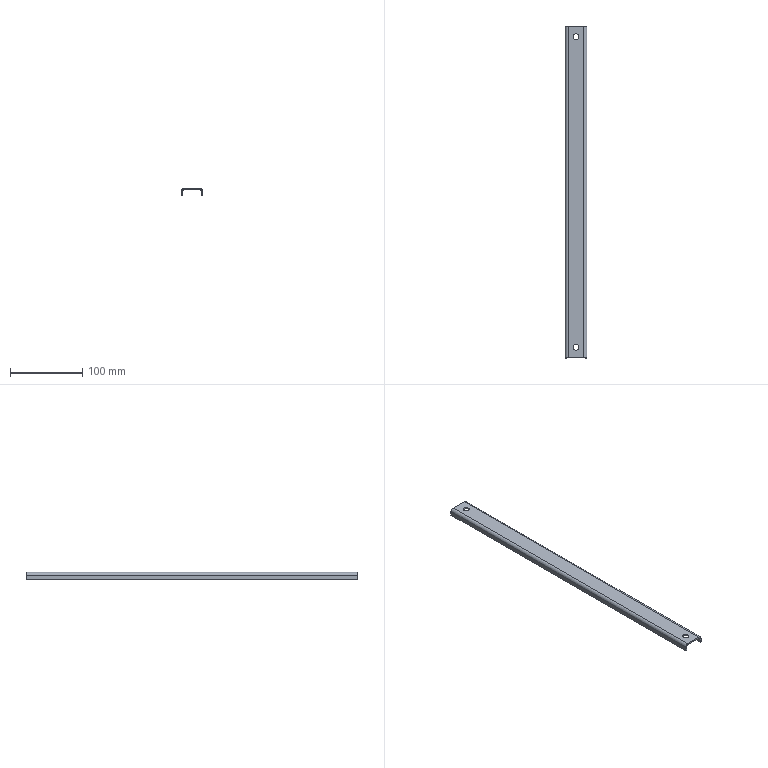Part | NX | features solid 2 | 1 solid | 18 faces | box 30 x 460 x 10 mm | volume 39740 mm3 | plane 10 | cylinder 8 | commonest cylinder face diameters 8.2 x4 4 x2 8 x2
STEP:
#1=CARTESIAN_POINT('',(690.9,502.5,-503.));
#2=VERTEX_POINT('',#1);
#3=CARTESIAN_POINT('',(690.9,502.5,-505.));
#4=VERTEX_POINT('',#3);
#5=CARTESIAN_POINT('',(690.9,502.5,-964.086));
#6=DIRECTION('',(0.,0.,1.));
#7=VECTOR('',#6,1000.);
#8=LINE('',#5,#7);
#9=EDGE_CURVE('',#2,#4,#8,.F.);
#10=ORIENTED_EDGE('',*,*,#9,.T.);
#11=CARTESIAN_POINT('',(699.1,502.5,-505.));
#12=VERTEX_POINT('',#11);
#13=CARTESIAN_POINT('',(695.,502.5,-505.));
#14=DIRECTION('',(0.,0.,-1.));
#15=DIRECTION('',(-1.,0.,0.));
#16=AXIS2_PLACEMENT_3D('',#13,#14,#15);
#17=CIRCLE('',#16,4.1);
#18=EDGE_CURVE('',#4,#12,#17,.T.);
#19=ORIENTED_EDGE('',*,*,#18,.T.);
#20=CARTESIAN_POINT('',(699.1,502.5,-503.));
#21=VERTEX_POINT('',#20);
#22=CARTESIAN_POINT('',(699.1,502.5,-964.086));
#23=DIRECTION('',(0.,0.,1.));
#24=VECTOR('',#23,1000.);
#25=LINE('',#22,#24);
#26=EDGE_CURVE('',#12,#21,#25,.T.);
#27=ORIENTED_EDGE('',*,*,#26,.T.);
#28=CARTESIAN_POINT('',(695.,502.5,-503.));
#29=DIRECTION('',(0.,0.,1.));
#30=DIRECTION('',(0.,1.,0.));
#31=AXIS2_PLACEMENT_3D('',#28,#29,#30);
#32=CIRCLE('',#31,4.1);
#33=EDGE_CURVE('',#21,#2,#32,.T.);
#34=ORIENTED_EDGE('',*,*,#33,.T.);
#35=EDGE_LOOP('',(#10,#19,#27,#34));
#36=FACE_BOUND('',#35,.T.);
#37=CARTESIAN_POINT('',(695.,502.5,-964.086));
#38=DIRECTION('',(0.,0.,1.));
#39=DIRECTION('',(1.,0.,0.));
#40=AXIS2_PLACEMENT_3D('',#37,#38,#39);
#41=CYLINDRICAL_SURFACE('',#40,4.1);
#42=ADVANCED_FACE('',(#36),#41,.F.);
#43=CARTESIAN_POINT('',(690.9,72.5,-505.));
#44=VERTEX_POINT('',#43);
#45=CARTESIAN_POINT('',(690.9,72.5,-503.));
#46=VERTEX_POINT('',#45);
#47=CARTESIAN_POINT('',(690.9,72.5,-964.086));
#48=DIRECTION('',(0.,0.,1.));
#49=VECTOR('',#48,1000.);
#50=LINE('',#47,#49);
#51=EDGE_CURVE('',#44,#46,#50,.T.);
#52=ORIENTED_EDGE('',*,*,#51,.F.);
#53=CARTESIAN_POINT('',(699.1,72.5,-505.));
#54=VERTEX_POINT('',#53);
#55=CARTESIAN_POINT('',(695.,72.5,-505.));
#56=DIRECTION('',(0.,0.,-1.));
#57=DIRECTION('',(-1.,0.,0.));
#58=AXIS2_PLACEMENT_3D('',#55,#56,#57);
#59=CIRCLE('',#58,4.1);
#60=EDGE_CURVE('',#44,#54,#59,.T.);
#61=ORIENTED_EDGE('',*,*,#60,.T.);
#62=CARTESIAN_POINT('',(699.1,72.5,-503.));
#63=VERTEX_POINT('',#62);
#64=CARTESIAN_POINT('',(699.1,72.5,-964.086));
#65=DIRECTION('',(0.,0.,1.));
#66=VECTOR('',#65,1000.);
#67=LINE('',#64,#66);
#68=EDGE_CURVE('',#63,#54,#67,.F.);
#69=ORIENTED_EDGE('',*,*,#68,.F.);
#70=CARTESIAN_POINT('',(695.,72.5,-503.));
#71=DIRECTION('',(0.,0.,1.));
#72=DIRECTION('',(0.,1.,0.));
#73=AXIS2_PLACEMENT_3D('',#70,#71,#72);
#74=CIRCLE('',#73,4.1);
#75=EDGE_CURVE('',#63,#46,#74,.T.);
#76=ORIENTED_EDGE('',*,*,#75,.T.);
#77=EDGE_LOOP('',(#52,#61,#69,#76));
#78=FACE_BOUND('',#77,.T.);
#79=CARTESIAN_POINT('',(695.,72.5,-964.086));
#80=DIRECTION('',(0.,0.,1.));
#81=DIRECTION('',(1.,0.,0.));
#82=AXIS2_PLACEMENT_3D('',#79,#80,#81);
#83=CYLINDRICAL_SURFACE('',#82,4.1);
#84=ADVANCED_FACE('',(#78),#83,.F.);
#85=CARTESIAN_POINT('',(680.,517.5,-507.));
#86=VERTEX_POINT('',#85);
#87=CARTESIAN_POINT('',(680.,517.5,-513.));
#88=VERTEX_POINT('',#87);
#89=CARTESIAN_POINT('',(680.,517.5,-503.));
#90=DIRECTION('',(0.,0.,-1.));
#91=VECTOR('',#90,1000.);
#92=LINE('',#89,#91);
#93=EDGE_CURVE('',#86,#88,#92,.T.);
#94=ORIENTED_EDGE('',*,*,#93,.T.);
#95=CARTESIAN_POINT('',(680.,57.5,-513.));
#96=VERTEX_POINT('',#95);
#97=CARTESIAN_POINT('',(680.,57.5,-513.));
#98=DIRECTION('',(0.,1.,0.));
#99=VECTOR('',#98,1000.);
#100=LINE('',#97,#99);
#101=EDGE_CURVE('',#96,#88,#100,.T.);
#102=ORIENTED_EDGE('',*,*,#101,.F.);
#103=CARTESIAN_POINT('',(680.,57.5,-507.));
#104=VERTEX_POINT('',#103);
#105=CARTESIAN_POINT('',(680.,57.5,-503.));
#106=DIRECTION('',(0.,0.,-1.));
#107=VECTOR('',#106,1000.);
#108=LINE('',#105,#107);
#109=EDGE_CURVE('',#104,#96,#108,.T.);
#110=ORIENTED_EDGE('',*,*,#109,.F.);
#111=CARTESIAN_POINT('',(680.,57.5,-507.));
#112=DIRECTION('',(0.,1.,0.));
#113=VECTOR('',#112,1000.);
#114=LINE('',#111,#113);
#115=EDGE_CURVE('',#104,#86,#114,.T.);
#116=ORIENTED_EDGE('',*,*,#115,.T.);
#117=EDGE_LOOP('',(#94,#102,#110,#116));
#118=FACE_BOUND('',#117,.T.);
#119=CARTESIAN_POINT('',(680.,57.5,-503.));
#120=DIRECTION('',(1.,0.,0.));
#121=DIRECTION('',(0.,-1.,0.));
#122=AXIS2_PLACEMENT_3D('',#119,#120,#121);
#123=PLANE('',#122);
#124=ADVANCED_FACE('',(#118),#123,.F.);
#125=CARTESIAN_POINT('',(684.,517.5,-503.));
#126=VERTEX_POINT('',#125);
#127=CARTESIAN_POINT('',(684.,517.5,-507.));
#128=DIRECTION('',(0.,-1.,0.));
#129=DIRECTION('',(0.,0.,1.));
#130=AXIS2_PLACEMENT_3D('',#127,#128,#129);
#131=CIRCLE('',#130,4.);
#132=EDGE_CURVE('',#126,#86,#131,.T.);
#133=ORIENTED_EDGE('',*,*,#132,.T.);
#134=ORIENTED_EDGE('',*,*,#115,.F.);
#135=CARTESIAN_POINT('',(684.,57.5,-503.));
#136=VERTEX_POINT('',#135);
#137=CARTESIAN_POINT('',(684.,57.5,-507.));
#138=DIRECTION('',(0.,-1.,0.));
#139=DIRECTION('',(0.,0.,1.));
#140=AXIS2_PLACEMENT_3D('',#137,#138,#139);
#141=CIRCLE('',#140,4.);
#142=EDGE_CURVE('',#136,#104,#141,.T.);
#143=ORIENTED_EDGE('',*,*,#142,.F.);
#144=CARTESIAN_POINT('',(684.,57.5,-503.));
#145=DIRECTION('',(0.,1.,0.));
#146=VECTOR('',#145,1000.);
#147=LINE('',#144,#146);
#148=EDGE_CURVE('',#136,#126,#147,.T.);
#149=ORIENTED_EDGE('',*,*,#148,.T.);
#150=EDGE_LOOP('',(#133,#134,#143,#149));
#151=FACE_BOUND('',#150,.T.);
#152=CARTESIAN_POINT('',(684.,57.5,-507.));
#153=DIRECTION('',(0.,1.,0.));
#154=DIRECTION('',(-1.,0.,0.));
#155=AXIS2_PLACEMENT_3D('',#152,#153,#154);
#156=CYLINDRICAL_SURFACE('',#155,4.);
#157=ADVANCED_FACE('',(#151),#156,.T.);
#158=ORIENTED_EDGE('',*,*,#75,.F.);
#159=CARTESIAN_POINT('',(695.,72.5,-503.));
#160=DIRECTION('',(0.,0.,1.));
#161=DIRECTION('',(0.,1.,0.));
#162=AXIS2_PLACEMENT_3D('',#159,#160,#161);
#163=CIRCLE('',#162,4.1);
#164=EDGE_CURVE('',#46,#63,#163,.T.);
#165=ORIENTED_EDGE('',*,*,#164,.F.);
#166=EDGE_LOOP('',(#158,#165));
#167=FACE_BOUND('',#166,.T.);
#168=ORIENTED_EDGE('',*,*,#33,.F.);
#169=CARTESIAN_POINT('',(695.,502.5,-503.));
#170=DIRECTION('',(0.,0.,1.));
#171=DIRECTION('',(0.,1.,0.));
#172=AXIS2_PLACEMENT_3D('',#169,#170,#171);
#173=CIRCLE('',#172,4.1);
#174=EDGE_CURVE('',#2,#21,#173,.T.);
#175=ORIENTED_EDGE('',*,*,#174,.F.);
#176=EDGE_LOOP('',(#168,#175));
#177=FACE_BOUND('',#176,.T.);
#178=CARTESIAN_POINT('',(706.,517.5,-503.));
#179=VERTEX_POINT('',#178);
#180=CARTESIAN_POINT('',(710.,517.5,-503.));
#181=DIRECTION('',(-1.,0.,0.));
#182=VECTOR('',#181,1000.);
#183=LINE('',#180,#182);
#184=EDGE_CURVE('',#179,#126,#183,.T.);
#185=ORIENTED_EDGE('',*,*,#184,.T.);
#186=ORIENTED_EDGE('',*,*,#148,.F.);
#187=CARTESIAN_POINT('',(706.,57.5,-503.));
#188=VERTEX_POINT('',#187);
#189=CARTESIAN_POINT('',(710.,57.5,-503.));
#190=DIRECTION('',(-1.,0.,0.));
#191=VECTOR('',#190,1000.);
#192=LINE('',#189,#191);
#193=EDGE_CURVE('',#188,#136,#192,.T.);
#194=ORIENTED_EDGE('',*,*,#193,.F.);
#195=CARTESIAN_POINT('',(706.,57.5,-503.));
#196=DIRECTION('',(0.,1.,0.));
#197=VECTOR('',#196,1000.);
#198=LINE('',#195,#197);
#199=EDGE_CURVE('',#188,#179,#198,.T.);
#200=ORIENTED_EDGE('',*,*,#199,.T.);
#201=EDGE_LOOP('',(#185,#186,#194,#200));
#202=FACE_BOUND('',#201,.T.);
#203=CARTESIAN_POINT('',(710.,57.5,-503.));
#204=DIRECTION('',(0.,0.,-1.));
#205=DIRECTION('',(-1.,0.,0.));
#206=AXIS2_PLACEMENT_3D('',#203,#204,#205);
#207=PLANE('',#206);
#208=ADVANCED_FACE('',(#167,#177,#202),#207,.F.);
#209=CARTESIAN_POINT('',(710.,517.5,-507.));
#210=VERTEX_POINT('',#209);
#211=CARTESIAN_POINT('',(706.,517.5,-507.));
#212=DIRECTION('',(0.,-1.,0.));
#213=DIRECTION('',(0.,0.,1.));
#214=AXIS2_PLACEMENT_3D('',#211,#212,#213);
#215=CIRCLE('',#214,4.);
#216=EDGE_CURVE('',#210,#179,#215,.T.);
#217=ORIENTED_EDGE('',*,*,#216,.T.);
#218=ORIENTED_EDGE('',*,*,#199,.F.);
#219=CARTESIAN_POINT('',(710.,57.5,-507.));
#220=VERTEX_POINT('',#219);
#221=CARTESIAN_POINT('',(706.,57.5,-507.));
#222=DIRECTION('',(0.,-1.,0.));
#223=DIRECTION('',(0.,0.,1.));
#224=AXIS2_PLACEMENT_3D('',#221,#222,#223);
#225=CIRCLE('',#224,4.);
#226=EDGE_CURVE('',#220,#188,#225,.T.);
#227=ORIENTED_EDGE('',*,*,#226,.F.);
#228=CARTESIAN_POINT('',(710.,57.5,-507.));
#229=DIRECTION('',(0.,1.,0.));
#230=VECTOR('',#229,1000.);
#231=LINE('',#228,#230);
#232=EDGE_CURVE('',#220,#210,#231,.T.);
#233=ORIENTED_EDGE('',*,*,#232,.T.);
#234=EDGE_LOOP('',(#217,#218,#227,#233));
#235=FACE_BOUND('',#234,.T.);
#236=CARTESIAN_POINT('',(706.,57.5,-507.));
#237=DIRECTION('',(0.,1.,0.));
#238=DIRECTION('',(-1.,0.,0.));
#239=AXIS2_PLACEMENT_3D('',#236,#237,#238);
#240=CYLINDRICAL_SURFACE('',#239,4.);
#241=ADVANCED_FACE('',(#235),#240,.T.);
#242=CARTESIAN_POINT('',(710.,517.5,-513.));
#243=VERTEX_POINT('',#242);
#244=CARTESIAN_POINT('',(710.,517.5,-513.));
#245=DIRECTION('',(0.,0.,1.));
#246=VECTOR('',#245,1000.);
#247=LINE('',#244,#246);
#248=EDGE_CURVE('',#243,#210,#247,.T.);
#249=ORIENTED_EDGE('',*,*,#248,.T.);
#250=ORIENTED_EDGE('',*,*,#232,.F.);
#251=CARTESIAN_POINT('',(710.,57.5,-513.));
#252=VERTEX_POINT('',#251);
#253=CARTESIAN_POINT('',(710.,57.5,-513.));
#254=DIRECTION('',(0.,0.,1.));
#255=VECTOR('',#254,1000.);
#256=LINE('',#253,#255);
#257=EDGE_CURVE('',#252,#220,#256,.T.);
#258=ORIENTED_EDGE('',*,*,#257,.F.);
#259=CARTESIAN_POINT('',(710.,57.5,-513.));
#260=DIRECTION('',(0.,1.,0.));
#261=VECTOR('',#260,1000.);
#262=LINE('',#259,#261);
#263=EDGE_CURVE('',#252,#243,#262,.T.);
#264=ORIENTED_EDGE('',*,*,#263,.T.);
#265=EDGE_LOOP('',(#249,#250,#258,#264));
#266=FACE_BOUND('',#265,.T.);
#267=CARTESIAN_POINT('',(710.,57.5,-513.));
#268=DIRECTION('',(-1.,0.,0.));
#269=DIRECTION('',(0.,0.,1.));
#270=AXIS2_PLACEMENT_3D('',#267,#268,#269);
#271=PLANE('',#270);
#272=ADVANCED_FACE('',(#266),#271,.F.);
#273=CARTESIAN_POINT('',(682.,517.5,-507.));
#274=VERTEX_POINT('',#273);
#275=CARTESIAN_POINT('',(682.,517.5,-513.));
#276=VERTEX_POINT('',#275);
#277=CARTESIAN_POINT('',(682.,517.5,-503.));
#278=DIRECTION('',(0.,0.,-1.));
#279=VECTOR('',#278,1000.);
#280=LINE('',#277,#279);
#281=EDGE_CURVE('',#274,#276,#280,.T.);
#282=ORIENTED_EDGE('',*,*,#281,.F.);
#283=CARTESIAN_POINT('',(682.,57.5,-507.));
#284=VERTEX_POINT('',#283);
#285=CARTESIAN_POINT('',(682.,57.5,-507.));
#286=DIRECTION('',(0.,1.,0.));
#287=VECTOR('',#286,1000.);
#288=LINE('',#285,#287);
#289=EDGE_CURVE('',#284,#274,#288,.T.);
#290=ORIENTED_EDGE('',*,*,#289,.F.);
#291=CARTESIAN_POINT('',(682.,57.5,-513.));
#292=VERTEX_POINT('',#291);
#293=CARTESIAN_POINT('',(682.,57.5,-503.));
#294=DIRECTION('',(0.,0.,-1.));
#295=VECTOR('',#294,1000.);
#296=LINE('',#293,#295);
#297=EDGE_CURVE('',#284,#292,#296,.T.);
#298=ORIENTED_EDGE('',*,*,#297,.T.);
#299=CARTESIAN_POINT('',(682.,57.5,-513.));
#300=DIRECTION('',(0.,1.,0.));
#301=VECTOR('',#300,1000.);
#302=LINE('',#299,#301);
#303=EDGE_CURVE('',#292,#276,#302,.T.);
#304=ORIENTED_EDGE('',*,*,#303,.T.);
#305=EDGE_LOOP('',(#282,#290,#298,#304));
#306=FACE_BOUND('',#305,.T.);
#307=CARTESIAN_POINT('',(682.,57.5,-503.));
#308=DIRECTION('',(1.,0.,0.));
#309=DIRECTION('',(0.,-1.,0.));
#310=AXIS2_PLACEMENT_3D('',#307,#308,#309);
#311=PLANE('',#310);
#312=ADVANCED_FACE('',(#306),#311,.T.);
#313=CARTESIAN_POINT('',(684.,517.5,-505.));
#314=VERTEX_POINT('',#313);
#315=CARTESIAN_POINT('',(684.,517.5,-507.));
#316=DIRECTION('',(0.,-1.,0.));
#317=DIRECTION('',(-1.,0.,0.));
#318=AXIS2_PLACEMENT_3D('',#315,#316,#317);
#319=CIRCLE('',#318,2.);
#320=EDGE_CURVE('',#314,#274,#319,.T.);
#321=ORIENTED_EDGE('',*,*,#320,.F.);
#322=CARTESIAN_POINT('',(684.,57.5,-505.));
#323=VERTEX_POINT('',#322);
#324=CARTESIAN_POINT('',(684.,57.5,-505.));
#325=DIRECTION('',(0.,1.,0.));
#326=VECTOR('',#325,1000.);
#327=LINE('',#324,#326);
#328=EDGE_CURVE('',#323,#314,#327,.T.);
#329=ORIENTED_EDGE('',*,*,#328,.F.);
#330=CARTESIAN_POINT('',(684.,57.5,-507.));
#331=DIRECTION('',(0.,-1.,0.));
#332=DIRECTION('',(-1.,0.,0.));
#333=AXIS2_PLACEMENT_3D('',#330,#331,#332);
#334=CIRCLE('',#333,2.);
#335=EDGE_CURVE('',#323,#284,#334,.T.);
#336=ORIENTED_EDGE('',*,*,#335,.T.);
#337=ORIENTED_EDGE('',*,*,#289,.T.);
#338=EDGE_LOOP('',(#321,#329,#336,#337));
#339=FACE_BOUND('',#338,.T.);
#340=CARTESIAN_POINT('',(684.,57.5,-507.));
#341=DIRECTION('',(0.,1.,0.));
#342=DIRECTION('',(-1.,0.,0.));
#343=AXIS2_PLACEMENT_3D('',#340,#341,#342);
#344=CYLINDRICAL_SURFACE('',#343,2.);
#345=ADVANCED_FACE('',(#339),#344,.F.);
#346=CARTESIAN_POINT('',(695.,72.5,-505.));
#347=DIRECTION('',(0.,0.,-1.));
#348=DIRECTION('',(-1.,0.,0.));
#349=AXIS2_PLACEMENT_3D('',#346,#347,#348);
#350=CIRCLE('',#349,4.1);
#351=EDGE_CURVE('',#54,#44,#350,.T.);
#352=ORIENTED_EDGE('',*,*,#351,.F.);
#353=ORIENTED_EDGE('',*,*,#60,.F.);
#354=EDGE_LOOP('',(#352,#353));
#355=FACE_BOUND('',#354,.T.);
#356=CARTESIAN_POINT('',(695.,502.5,-505.));
#357=DIRECTION('',(0.,0.,-1.));
#358=DIRECTION('',(-1.,0.,0.));
#359=AXIS2_PLACEMENT_3D('',#356,#357,#358);
#360=CIRCLE('',#359,4.1);
#361=EDGE_CURVE('',#12,#4,#360,.T.);
#362=ORIENTED_EDGE('',*,*,#361,.F.);
#363=ORIENTED_EDGE('',*,*,#18,.F.);
#364=EDGE_LOOP('',(#362,#363));
#365=FACE_BOUND('',#364,.T.);
#366=CARTESIAN_POINT('',(706.,517.5,-505.));
#367=VERTEX_POINT('',#366);
#368=CARTESIAN_POINT('',(710.,517.5,-505.));
#369=DIRECTION('',(-1.,0.,0.));
#370=VECTOR('',#369,1000.);
#371=LINE('',#368,#370);
#372=EDGE_CURVE('',#367,#314,#371,.T.);
#373=ORIENTED_EDGE('',*,*,#372,.F.);
#374=CARTESIAN_POINT('',(706.,57.5,-505.));
#375=VERTEX_POINT('',#374);
#376=CARTESIAN_POINT('',(706.,57.5,-505.));
#377=DIRECTION('',(0.,1.,0.));
#378=VECTOR('',#377,1000.);
#379=LINE('',#376,#378);
#380=EDGE_CURVE('',#375,#367,#379,.T.);
#381=ORIENTED_EDGE('',*,*,#380,.F.);
#382=CARTESIAN_POINT('',(710.,57.5,-505.));
#383=DIRECTION('',(-1.,0.,0.));
#384=VECTOR('',#383,1000.);
#385=LINE('',#382,#384);
#386=EDGE_CURVE('',#375,#323,#385,.T.);
#387=ORIENTED_EDGE('',*,*,#386,.T.);
#388=ORIENTED_EDGE('',*,*,#328,.T.);
#389=EDGE_LOOP('',(#373,#381,#387,#388));
#390=FACE_BOUND('',#389,.T.);
#391=CARTESIAN_POINT('',(710.,57.5,-505.));
#392=DIRECTION('',(0.,0.,-1.));
#393=DIRECTION('',(-1.,0.,0.));
#394=AXIS2_PLACEMENT_3D('',#391,#392,#393);
#395=PLANE('',#394);
#396=ADVANCED_FACE('',(#355,#365,#390),#395,.T.);
#397=CARTESIAN_POINT('',(708.,517.5,-507.));
#398=VERTEX_POINT('',#397);
#399=CARTESIAN_POINT('',(706.,517.5,-507.));
#400=DIRECTION('',(0.,-1.,0.));
#401=DIRECTION('',(-1.,0.,0.));
#402=AXIS2_PLACEMENT_3D('',#399,#400,#401);
#403=CIRCLE('',#402,2.);
#404=EDGE_CURVE('',#398,#367,#403,.T.);
#405=ORIENTED_EDGE('',*,*,#404,.F.);
#406=CARTESIAN_POINT('',(708.,57.5,-507.));
#407=VERTEX_POINT('',#406);
#408=CARTESIAN_POINT('',(708.,57.5,-507.));
#409=DIRECTION('',(0.,1.,0.));
#410=VECTOR('',#409,1000.);
#411=LINE('',#408,#410);
#412=EDGE_CURVE('',#407,#398,#411,.T.);
#413=ORIENTED_EDGE('',*,*,#412,.F.);
#414=CARTESIAN_POINT('',(706.,57.5,-507.));
#415=DIRECTION('',(0.,-1.,0.));
#416=DIRECTION('',(-1.,0.,0.));
#417=AXIS2_PLACEMENT_3D('',#414,#415,#416);
#418=CIRCLE('',#417,2.);
#419=EDGE_CURVE('',#407,#375,#418,.T.);
#420=ORIENTED_EDGE('',*,*,#419,.T.);
#421=ORIENTED_EDGE('',*,*,#380,.T.);
#422=EDGE_LOOP('',(#405,#413,#420,#421));
#423=FACE_BOUND('',#422,.T.);
#424=CARTESIAN_POINT('',(706.,57.5,-507.));
#425=DIRECTION('',(0.,1.,0.));
#426=DIRECTION('',(-1.,0.,0.));
#427=AXIS2_PLACEMENT_3D('',#424,#425,#426);
#428=CYLINDRICAL_SURFACE('',#427,2.);
#429=ADVANCED_FACE('',(#423),#428,.F.);
#430=CARTESIAN_POINT('',(708.,517.5,-513.));
#431=VERTEX_POINT('',#430);
#432=CARTESIAN_POINT('',(708.,517.5,-513.));
#433=DIRECTION('',(0.,0.,1.));
#434=VECTOR('',#433,1000.);
#435=LINE('',#432,#434);
#436=EDGE_CURVE('',#431,#398,#435,.T.);
#437=ORIENTED_EDGE('',*,*,#436,.F.);
#438=CARTESIAN_POINT('',(708.,57.5,-513.));
#439=VERTEX_POINT('',#438);
#440=CARTESIAN_POINT('',(708.,57.5,-513.));
#441=DIRECTION('',(0.,1.,0.));
#442=VECTOR('',#441,1000.);
#443=LINE('',#440,#442);
#444=EDGE_CURVE('',#439,#431,#443,.T.);
#445=ORIENTED_EDGE('',*,*,#444,.F.);
#446=CARTESIAN_POINT('',(708.,57.5,-513.));
#447=DIRECTION('',(0.,0.,1.));
#448=VECTOR('',#447,1000.);
#449=LINE('',#446,#448);
#450=EDGE_CURVE('',#439,#407,#449,.T.);
#451=ORIENTED_EDGE('',*,*,#450,.T.);
#452=ORIENTED_EDGE('',*,*,#412,.T.);
#453=EDGE_LOOP('',(#437,#445,#451,#452));
#454=FACE_BOUND('',#453,.T.);
#455=CARTESIAN_POINT('',(708.,57.5,-513.));
#456=DIRECTION('',(-1.,0.,0.));
#457=DIRECTION('',(0.,0.,1.));
#458=AXIS2_PLACEMENT_3D('',#455,#456,#457);
#459=PLANE('',#458);
#460=ADVANCED_FACE('',(#454),#459,.T.);
#461=ORIENTED_EDGE('',*,*,#263,.F.);
#462=CARTESIAN_POINT('',(710.,57.5,-513.));
#463=DIRECTION('',(-1.,0.,0.));
#464=VECTOR('',#463,1000.);
#465=LINE('',#462,#464);
#466=EDGE_CURVE('',#252,#439,#465,.T.);
#467=ORIENTED_EDGE('',*,*,#466,.T.);
#468=ORIENTED_EDGE('',*,*,#444,.T.);
#469=CARTESIAN_POINT('',(710.,517.5,-513.));
#470=DIRECTION('',(-1.,0.,0.));
#471=VECTOR('',#470,1000.);
#472=LINE('',#469,#471);
#473=EDGE_CURVE('',#243,#431,#472,.T.);
#474=ORIENTED_EDGE('',*,*,#473,.F.);
#475=EDGE_LOOP('',(#461,#467,#468,#474));
#476=FACE_BOUND('',#475,.T.);
#477=CARTESIAN_POINT('',(710.,57.5,-513.));
#478=DIRECTION('',(0.,0.,1.));
#479=DIRECTION('',(0.,-1.,0.));
#480=AXIS2_PLACEMENT_3D('',#477,#478,#479);
#481=PLANE('',#480);
#482=ADVANCED_FACE('',(#476),#481,.F.);
#483=ORIENTED_EDGE('',*,*,#436,.T.);
#484=ORIENTED_EDGE('',*,*,#404,.T.);
#485=ORIENTED_EDGE('',*,*,#372,.T.);
#486=ORIENTED_EDGE('',*,*,#320,.T.);
#487=ORIENTED_EDGE('',*,*,#281,.T.);
#488=CARTESIAN_POINT('',(680.,517.5,-513.));
#489=DIRECTION('',(1.,0.,0.));
#490=VECTOR('',#489,1000.);
#491=LINE('',#488,#490);
#492=EDGE_CURVE('',#88,#276,#491,.T.);
#493=ORIENTED_EDGE('',*,*,#492,.F.);
#494=ORIENTED_EDGE('',*,*,#93,.F.);
#495=ORIENTED_EDGE('',*,*,#132,.F.);
#496=ORIENTED_EDGE('',*,*,#184,.F.);
#497=ORIENTED_EDGE('',*,*,#216,.F.);
#498=ORIENTED_EDGE('',*,*,#248,.F.);
#499=ORIENTED_EDGE('',*,*,#473,.T.);
#500=EDGE_LOOP('',(#483,#484,#485,#486,#487,#493,#494,#495,#496,#497,#498,#499));
#501=FACE_BOUND('',#500,.T.);
#502=CARTESIAN_POINT('',(710.,517.5,-513.));
#503=DIRECTION('',(0.,-1.,0.));
#504=DIRECTION('',(-1.,0.,0.));
#505=AXIS2_PLACEMENT_3D('',#502,#503,#504);
#506=PLANE('',#505);
#507=ADVANCED_FACE('',(#501),#506,.F.);
#508=CARTESIAN_POINT('',(680.,57.5,-513.));
#509=DIRECTION('',(1.,0.,0.));
#510=VECTOR('',#509,1000.);
#511=LINE('',#508,#510);
#512=EDGE_CURVE('',#96,#292,#511,.T.);
#513=ORIENTED_EDGE('',*,*,#512,.F.);
#514=ORIENTED_EDGE('',*,*,#101,.T.);
#515=ORIENTED_EDGE('',*,*,#492,.T.);
#516=ORIENTED_EDGE('',*,*,#303,.F.);
#517=EDGE_LOOP('',(#513,#514,#515,#516));
#518=FACE_BOUND('',#517,.T.);
#519=CARTESIAN_POINT('',(680.,57.5,-513.));
#520=DIRECTION('',(0.,0.,-1.));
#521=DIRECTION('',(-1.,0.,0.));
#522=AXIS2_PLACEMENT_3D('',#519,#520,#521);
#523=PLANE('',#522);
#524=ADVANCED_FACE('',(#518),#523,.T.);
#525=ORIENTED_EDGE('',*,*,#297,.F.);
#526=ORIENTED_EDGE('',*,*,#335,.F.);
#527=ORIENTED_EDGE('',*,*,#386,.F.);
#528=ORIENTED_EDGE('',*,*,#419,.F.);
#529=ORIENTED_EDGE('',*,*,#450,.F.);
#530=ORIENTED_EDGE('',*,*,#466,.F.);
#531=ORIENTED_EDGE('',*,*,#257,.T.);
#532=ORIENTED_EDGE('',*,*,#226,.T.);
#533=ORIENTED_EDGE('',*,*,#193,.T.);
#534=ORIENTED_EDGE('',*,*,#142,.T.);
#535=ORIENTED_EDGE('',*,*,#109,.T.);
#536=ORIENTED_EDGE('',*,*,#512,.T.);
#537=EDGE_LOOP('',(#525,#526,#527,#528,#529,#530,#531,#532,#533,#534,#535,#536));
#538=FACE_BOUND('',#537,.T.);
#539=CARTESIAN_POINT('',(680.,57.5,-503.));
#540=DIRECTION('',(0.,-1.,0.));
#541=DIRECTION('',(-1.,0.,0.));
#542=AXIS2_PLACEMENT_3D('',#539,#540,#541);
#543=PLANE('',#542);
#544=ADVANCED_FACE('',(#538),#543,.T.);
#545=ORIENTED_EDGE('',*,*,#351,.T.);
#546=ORIENTED_EDGE('',*,*,#51,.T.);
#547=ORIENTED_EDGE('',*,*,#164,.T.);
#548=ORIENTED_EDGE('',*,*,#68,.T.);
#549=EDGE_LOOP('',(#545,#546,#547,#548));
#550=FACE_BOUND('',#549,.T.);
#551=CARTESIAN_POINT('',(695.,72.5,-964.086));
#552=DIRECTION('',(0.,0.,1.));
#553=DIRECTION('',(1.,0.,0.));
#554=AXIS2_PLACEMENT_3D('',#551,#552,#553);
#555=CYLINDRICAL_SURFACE('',#554,4.1);
#556=ADVANCED_FACE('',(#550),#555,.F.);
#557=ORIENTED_EDGE('',*,*,#361,.T.);
#558=ORIENTED_EDGE('',*,*,#9,.F.);
#559=ORIENTED_EDGE('',*,*,#174,.T.);
#560=ORIENTED_EDGE('',*,*,#26,.F.);
#561=EDGE_LOOP('',(#557,#558,#559,#560));
#562=FACE_BOUND('',#561,.T.);
#563=CARTESIAN_POINT('',(695.,502.5,-964.086));
#564=DIRECTION('',(0.,0.,1.));
#565=DIRECTION('',(1.,0.,0.));
#566=AXIS2_PLACEMENT_3D('',#563,#564,#565);
#567=CYLINDRICAL_SURFACE('',#566,4.1);
#568=ADVANCED_FACE('',(#562),#567,.F.);
#569=CLOSED_SHELL('',(#42,#84,#124,#157,#208,#241,#272,#312,#345,#396,#429,#460,#482,#507,#524,#544,#556,#568));
#570=MANIFOLD_SOLID_BREP('',#569);
#571=(LENGTH_UNIT()NAMED_UNIT(*)SI_UNIT(.MILLI.,.METRE.));
#572=UNCERTAINTY_MEASURE_WITH_UNIT(LENGTH_MEASURE(0.00001),#571,'','');
#573=(NAMED_UNIT(*)PLANE_ANGLE_UNIT()SI_UNIT($,.RADIAN.));
#574=(NAMED_UNIT(*)SI_UNIT($,.STERADIAN.)SOLID_ANGLE_UNIT());
#575=(GEOMETRIC_REPRESENTATION_CONTEXT(3)GLOBAL_UNCERTAINTY_ASSIGNED_CONTEXT((#572))GLOBAL_UNIT_ASSIGNED_CONTEXT((#571,#573,#574))REPRESENTATION_CONTEXT('',''));
#576=ADVANCED_BREP_SHAPE_REPRESENTATION('',(#570),#575);